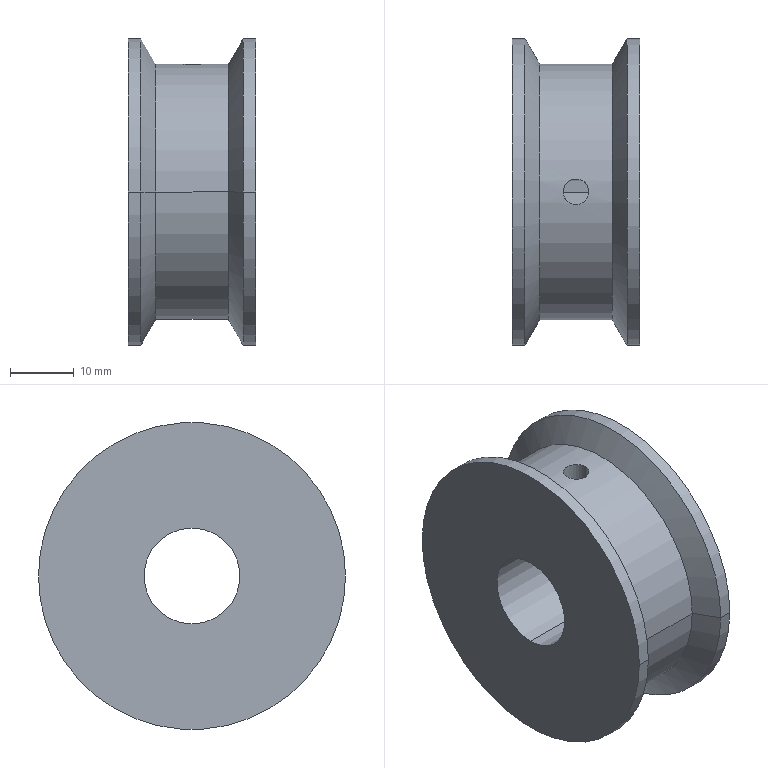Part | SolidWorks | features BaseBody 1 | 1 solid | 16 faces | box 20 x 48 x 48 mm | volume 24891 mm3 | cylinder 10 | cone 4 | plane 2 | commonest cylinder face diameters 48 x4 4 x2 15 x2 40 x2
STEP:
#1=CARTESIAN_POINT('',(2.,0.,7.5));
#2=VERTEX_POINT('',#1);
#3=CARTESIAN_POINT('',(-2.,0.,7.5));
#4=VERTEX_POINT('',#3);
#5=CARTESIAN_POINT('',(2.,0.,7.5));
#6=CARTESIAN_POINT('',(2.,0.1327,7.5));
#7=CARTESIAN_POINT('',(1.987,0.2632,7.496));
#8=CARTESIAN_POINT('',(1.936,0.5196,7.483));
#9=CARTESIAN_POINT('',(1.897,0.6469,7.473));
#10=CARTESIAN_POINT('',(1.796,0.8888,7.448));
#11=CARTESIAN_POINT('',(1.735,1.003,7.433));
#12=CARTESIAN_POINT('',(1.59,1.22,7.401));
#13=CARTESIAN_POINT('',(1.506,1.323,7.383));
#14=CARTESIAN_POINT('',(1.231,1.598,7.33));
#15=CARTESIAN_POINT('',(1.009,1.747,7.295));
#16=CARTESIAN_POINT('',(0.6481,1.897,7.256));
#17=CARTESIAN_POINT('',(0.5215,1.935,7.246));
#18=CARTESIAN_POINT('',(0.2631,1.987,7.232));
#19=CARTESIAN_POINT('',(0.1329,2.,7.228));
#20=CARTESIAN_POINT('',(-0.1292,2.,7.228));
#21=CARTESIAN_POINT('',(-0.2624,1.987,7.232));
#22=CARTESIAN_POINT('',(-0.5194,1.936,7.246));
#23=CARTESIAN_POINT('',(-0.6443,1.898,7.256));
#24=CARTESIAN_POINT('',(-1.009,1.747,7.294));
#25=CARTESIAN_POINT('',(-1.228,1.6,7.33));
#26=CARTESIAN_POINT('',(-1.506,1.322,7.383));
#27=CARTESIAN_POINT('',(-1.588,1.222,7.401));
#28=CARTESIAN_POINT('',(-1.733,1.006,7.433));
#29=CARTESIAN_POINT('',(-1.796,0.8891,7.448));
#30=CARTESIAN_POINT('',(-1.897,0.6479,7.473));
#31=CARTESIAN_POINT('',(-1.935,0.5233,7.483));
#32=CARTESIAN_POINT('',(-1.987,0.2656,7.496));
#33=CARTESIAN_POINT('',(-2.,0.1328,7.5));
#34=CARTESIAN_POINT('',(-2.,0.,7.5));
#35=B_SPLINE_CURVE_WITH_KNOTS('',3,(#5,#6,#7,#8,#9,#10,#11,#12,#13,#14,#15,#16,#17,#18,#19,#20,#21,#22,#23,#24,#25,#26,#27,#28,#29,#30,#31,#32,#33,#34),.UNSPECIFIED.,.F.,.F.,(4,2,2,2,2,2,2,2,2,2,2,2,2,2,4),(0.,0.0003925,0.0007849,0.001177,0.00157,0.002355,0.002747,0.00314,0.003532,0.003925,0.00471,0.005102,0.005495,0.005887,0.006279),.UNSPECIFIED.);
#36=EDGE_CURVE('',#2,#4,#35,.T.);
#37=ORIENTED_EDGE('',*,*,#36,.F.);
#38=CARTESIAN_POINT('',(2.,0.,20.));
#39=VERTEX_POINT('',#38);
#40=CARTESIAN_POINT('',(2.,0.,20.));
#41=DIRECTION('',(0.,0.,1.));
#42=VECTOR('',#41,1000.);
#43=LINE('',#40,#42);
#44=EDGE_CURVE('',#2,#39,#43,.T.);
#45=ORIENTED_EDGE('',*,*,#44,.T.);
#46=CARTESIAN_POINT('',(-2.,0.,20.));
#47=VERTEX_POINT('',#46);
#48=CARTESIAN_POINT('',(-2.,0.,20.));
#49=CARTESIAN_POINT('',(-2.,0.1322,20.));
#50=CARTESIAN_POINT('',(-1.987,0.2622,19.999));
#51=CARTESIAN_POINT('',(-1.936,0.5179,19.994));
#52=CARTESIAN_POINT('',(-1.898,0.6449,19.99));
#53=CARTESIAN_POINT('',(-1.797,0.8871,19.981));
#54=CARTESIAN_POINT('',(-1.736,1.002,19.975));
#55=CARTESIAN_POINT('',(-1.591,1.219,19.963));
#56=CARTESIAN_POINT('',(-1.506,1.322,19.956));
#57=CARTESIAN_POINT('',(-1.23,1.599,19.937));
#58=CARTESIAN_POINT('',(-1.007,1.748,19.924));
#59=CARTESIAN_POINT('',(-0.5257,1.947,19.905));
#60=CARTESIAN_POINT('',(-0.2624,2.,19.9));
#61=CARTESIAN_POINT('',(0.1291,2.,19.9));
#62=CARTESIAN_POINT('',(0.2617,1.987,19.901));
#63=CARTESIAN_POINT('',(0.5182,1.936,19.906));
#64=CARTESIAN_POINT('',(0.6429,1.898,19.91));
#65=CARTESIAN_POINT('',(0.8851,1.798,19.919));
#66=CARTESIAN_POINT('',(1.002,1.736,19.925));
#67=CARTESIAN_POINT('',(1.219,1.591,19.937));
#68=CARTESIAN_POINT('',(1.32,1.508,19.943));
#69=CARTESIAN_POINT('',(1.507,1.322,19.956));
#70=CARTESIAN_POINT('',(1.589,1.221,19.963));
#71=CARTESIAN_POINT('',(1.734,1.005,19.975));
#72=CARTESIAN_POINT('',(1.797,0.8877,19.981));
#73=CARTESIAN_POINT('',(1.897,0.6455,19.99));
#74=CARTESIAN_POINT('',(1.935,0.5209,19.994));
#75=CARTESIAN_POINT('',(1.987,0.2645,19.999));
#76=CARTESIAN_POINT('',(2.,0.1322,20.));
#77=CARTESIAN_POINT('',(2.,0.,20.));
#78=B_SPLINE_CURVE_WITH_KNOTS('',3,(#48,#49,#50,#51,#52,#53,#54,#55,#56,#57,#58,#59,#60,#61,#62,#63,#64,#65,#66,#67,#68,#69,#70,#71,#72,#73,#74,#75,#76,#77),.UNSPECIFIED.,.F.,.F.,(4,2,2,2,2,2,2,2,2,2,2,2,2,2,4),(0.,0.000391,0.0007819,0.001173,0.001564,0.002346,0.003128,0.003519,0.00391,0.004301,0.004692,0.005083,0.005474,0.005864,0.006255),.UNSPECIFIED.);
#79=EDGE_CURVE('',#47,#39,#78,.T.);
#80=ORIENTED_EDGE('',*,*,#79,.F.);
#81=CARTESIAN_POINT('',(-2.,0.,20.));
#82=DIRECTION('',(0.,0.,1.));
#83=VECTOR('',#82,1000.);
#84=LINE('',#81,#83);
#85=EDGE_CURVE('',#4,#47,#84,.T.);
#86=ORIENTED_EDGE('',*,*,#85,.F.);
#87=EDGE_LOOP('',(#37,#45,#80,#86));
#88=FACE_OUTER_BOUND('',#87,.T.);
#89=CARTESIAN_POINT('',(0.,0.,20.));
#90=DIRECTION('',(0.,0.,1.));
#91=DIRECTION('',(-1.,0.,0.));
#92=AXIS2_PLACEMENT_3D('',#89,#90,#91);
#93=CYLINDRICAL_SURFACE('',#92,2.);
#94=ADVANCED_FACE('',(#88),#93,.F.);
#95=CARTESIAN_POINT('',(-10.,0.,-7.5));
#96=VERTEX_POINT('',#95);
#97=CARTESIAN_POINT('',(-10.,0.,7.5));
#98=VERTEX_POINT('',#97);
#99=CARTESIAN_POINT('',(-10.,0.,0.));
#100=DIRECTION('',(1.,0.,0.));
#101=DIRECTION('',(0.,0.,1.));
#102=AXIS2_PLACEMENT_3D('',#99,#100,#101);
#103=CIRCLE('',#102,7.5);
#104=EDGE_CURVE('',#96,#98,#103,.T.);
#105=ORIENTED_EDGE('',*,*,#104,.F.);
#106=CARTESIAN_POINT('',(10.,0.,-7.5));
#107=VERTEX_POINT('',#106);
#108=CARTESIAN_POINT('',(10.,0.,-7.5));
#109=DIRECTION('',(1.,0.,0.));
#110=VECTOR('',#109,1000.);
#111=LINE('',#108,#110);
#112=EDGE_CURVE('',#96,#107,#111,.T.);
#113=ORIENTED_EDGE('',*,*,#112,.T.);
#114=CARTESIAN_POINT('',(10.,0.,7.5));
#115=VERTEX_POINT('',#114);
#116=CARTESIAN_POINT('',(10.,0.,0.));
#117=DIRECTION('',(-1.,0.,0.));
#118=DIRECTION('',(0.,0.,1.));
#119=AXIS2_PLACEMENT_3D('',#116,#117,#118);
#120=CIRCLE('',#119,7.5);
#121=EDGE_CURVE('',#115,#107,#120,.T.);
#122=ORIENTED_EDGE('',*,*,#121,.F.);
#123=CARTESIAN_POINT('',(10.,0.,7.5));
#124=DIRECTION('',(1.,0.,0.));
#125=VECTOR('',#124,1000.);
#126=LINE('',#123,#125);
#127=EDGE_CURVE('',#2,#115,#126,.T.);
#128=ORIENTED_EDGE('',*,*,#127,.F.);
#129=ORIENTED_EDGE('',*,*,#36,.T.);
#130=CARTESIAN_POINT('',(10.,0.,7.5));
#131=DIRECTION('',(1.,0.,0.));
#132=VECTOR('',#131,1000.);
#133=LINE('',#130,#132);
#134=EDGE_CURVE('',#98,#4,#133,.T.);
#135=ORIENTED_EDGE('',*,*,#134,.F.);
#136=EDGE_LOOP('',(#105,#113,#122,#128,#129,#135));
#137=FACE_OUTER_BOUND('',#136,.T.);
#138=CARTESIAN_POINT('',(10.,0.,0.));
#139=DIRECTION('',(1.,0.,0.));
#140=DIRECTION('',(0.,0.,1.));
#141=AXIS2_PLACEMENT_3D('',#138,#139,#140);
#142=CYLINDRICAL_SURFACE('',#141,7.5);
#143=ADVANCED_FACE('',(#137),#142,.F.);
#144=CARTESIAN_POINT('',(-8.,-24.,0.));
#145=VERTEX_POINT('',#144);
#146=CARTESIAN_POINT('',(-8.,24.,0.));
#147=VERTEX_POINT('',#146);
#148=CARTESIAN_POINT('',(-8.,0.,0.));
#149=DIRECTION('',(1.,0.,0.));
#150=DIRECTION('',(0.,0.,-1.));
#151=AXIS2_PLACEMENT_3D('',#148,#149,#150);
#152=CIRCLE('',#151,24.);
#153=EDGE_CURVE('',#145,#147,#152,.T.);
#154=ORIENTED_EDGE('',*,*,#153,.F.);
#155=CARTESIAN_POINT('',(-10.,-24.,0.));
#156=VERTEX_POINT('',#155);
#157=CARTESIAN_POINT('',(-9.,-24.,0.));
#158=DIRECTION('',(-1.,0.,0.));
#159=VECTOR('',#158,1000.);
#160=LINE('',#157,#159);
#161=EDGE_CURVE('',#145,#156,#160,.T.);
#162=ORIENTED_EDGE('',*,*,#161,.T.);
#163=CARTESIAN_POINT('',(-10.,24.,0.));
#164=VERTEX_POINT('',#163);
#165=CARTESIAN_POINT('',(-10.,0.,0.));
#166=DIRECTION('',(1.,0.,0.));
#167=DIRECTION('',(0.,0.,-1.));
#168=AXIS2_PLACEMENT_3D('',#165,#166,#167);
#169=CIRCLE('',#168,24.);
#170=EDGE_CURVE('',#156,#164,#169,.T.);
#171=ORIENTED_EDGE('',*,*,#170,.T.);
#172=CARTESIAN_POINT('',(-9.,24.,0.));
#173=DIRECTION('',(-1.,0.,0.));
#174=VECTOR('',#173,1000.);
#175=LINE('',#172,#174);
#176=EDGE_CURVE('',#147,#164,#175,.T.);
#177=ORIENTED_EDGE('',*,*,#176,.F.);
#178=EDGE_LOOP('',(#154,#162,#171,#177));
#179=FACE_OUTER_BOUND('',#178,.T.);
#180=CARTESIAN_POINT('',(-9.,0.,0.));
#181=DIRECTION('',(-1.,0.,0.));
#182=DIRECTION('',(0.,1.,0.));
#183=AXIS2_PLACEMENT_3D('',#180,#181,#182);
#184=CYLINDRICAL_SURFACE('',#183,24.);
#185=ADVANCED_FACE('',(#179),#184,.T.);
#186=CARTESIAN_POINT('',(-5.691,-20.,0.));
#187=VERTEX_POINT('',#186);
#188=CARTESIAN_POINT('',(-5.691,20.,0.));
#189=VERTEX_POINT('',#188);
#190=CARTESIAN_POINT('',(-5.691,0.,0.));
#191=DIRECTION('',(1.,0.,0.));
#192=DIRECTION('',(0.,0.,-1.));
#193=AXIS2_PLACEMENT_3D('',#190,#191,#192);
#194=CIRCLE('',#193,20.);
#195=EDGE_CURVE('',#187,#189,#194,.T.);
#196=ORIENTED_EDGE('',*,*,#195,.F.);
#197=CARTESIAN_POINT('',(-6.845,-22.,0.));
#198=DIRECTION('',(-0.5,-0.866,0.));
#199=VECTOR('',#198,1000.);
#200=LINE('',#197,#199);
#201=EDGE_CURVE('',#187,#145,#200,.T.);
#202=ORIENTED_EDGE('',*,*,#201,.T.);
#203=ORIENTED_EDGE('',*,*,#153,.T.);
#204=CARTESIAN_POINT('',(-6.845,22.,0.));
#205=DIRECTION('',(-0.5,0.866,0.));
#206=VECTOR('',#205,1000.);
#207=LINE('',#204,#206);
#208=EDGE_CURVE('',#189,#147,#207,.T.);
#209=ORIENTED_EDGE('',*,*,#208,.F.);
#210=EDGE_LOOP('',(#196,#202,#203,#209));
#211=FACE_OUTER_BOUND('',#210,.T.);
#212=CARTESIAN_POINT('',(-6.845,0.,0.));
#213=DIRECTION('',(-1.,0.,0.));
#214=DIRECTION('',(0.,1.,0.));
#215=AXIS2_PLACEMENT_3D('',#212,#213,#214);
#216=CONICAL_SURFACE('',#215,22.,1.047);
#217=ADVANCED_FACE('',(#211),#216,.T.);
#218=CARTESIAN_POINT('',(5.691,-20.,0.));
#219=VERTEX_POINT('',#218);
#220=CARTESIAN_POINT('',(5.691,20.,0.));
#221=VERTEX_POINT('',#220);
#222=CARTESIAN_POINT('',(5.691,0.,0.));
#223=DIRECTION('',(1.,0.,0.));
#224=DIRECTION('',(0.,0.,-1.));
#225=AXIS2_PLACEMENT_3D('',#222,#223,#224);
#226=CIRCLE('',#225,20.);
#227=EDGE_CURVE('',#219,#221,#226,.T.);
#228=ORIENTED_EDGE('',*,*,#227,.F.);
#229=CARTESIAN_POINT('',(0.,-20.,0.));
#230=DIRECTION('',(-1.,0.,0.));
#231=VECTOR('',#230,1000.);
#232=LINE('',#229,#231);
#233=EDGE_CURVE('',#219,#187,#232,.T.);
#234=ORIENTED_EDGE('',*,*,#233,.T.);
#235=ORIENTED_EDGE('',*,*,#195,.T.);
#236=CARTESIAN_POINT('',(0.,20.,0.));
#237=DIRECTION('',(-1.,0.,0.));
#238=VECTOR('',#237,1000.);
#239=LINE('',#236,#238);
#240=EDGE_CURVE('',#221,#189,#239,.T.);
#241=ORIENTED_EDGE('',*,*,#240,.F.);
#242=EDGE_LOOP('',(#228,#234,#235,#241));
#243=FACE_OUTER_BOUND('',#242,.T.);
#244=CARTESIAN_POINT('',(0.,0.,0.));
#245=DIRECTION('',(-1.,0.,0.));
#246=DIRECTION('',(0.,1.,0.));
#247=AXIS2_PLACEMENT_3D('',#244,#245,#246);
#248=CYLINDRICAL_SURFACE('',#247,20.);
#249=ADVANCED_FACE('',(#243),#248,.T.);
#250=CARTESIAN_POINT('',(5.691,0.,0.));
#251=DIRECTION('',(1.,0.,0.));
#252=DIRECTION('',(0.,0.,-1.));
#253=AXIS2_PLACEMENT_3D('',#250,#251,#252);
#254=CIRCLE('',#253,20.);
#255=EDGE_CURVE('',#221,#219,#254,.T.);
#256=ORIENTED_EDGE('',*,*,#255,.T.);
#257=CARTESIAN_POINT('',(8.,-24.,0.));
#258=VERTEX_POINT('',#257);
#259=CARTESIAN_POINT('',(6.845,-22.,0.));
#260=DIRECTION('',(0.5,-0.866,0.));
#261=VECTOR('',#260,1000.);
#262=LINE('',#259,#261);
#263=EDGE_CURVE('',#219,#258,#262,.T.);
#264=ORIENTED_EDGE('',*,*,#263,.T.);
#265=CARTESIAN_POINT('',(8.,24.,0.));
#266=VERTEX_POINT('',#265);
#267=CARTESIAN_POINT('',(8.,0.,0.));
#268=DIRECTION('',(1.,0.,0.));
#269=DIRECTION('',(0.,0.,-1.));
#270=AXIS2_PLACEMENT_3D('',#267,#268,#269);
#271=CIRCLE('',#270,24.);
#272=EDGE_CURVE('',#266,#258,#271,.T.);
#273=ORIENTED_EDGE('',*,*,#272,.F.);
#274=CARTESIAN_POINT('',(6.845,22.,0.));
#275=DIRECTION('',(0.5,0.866,0.));
#276=VECTOR('',#275,1000.);
#277=LINE('',#274,#276);
#278=EDGE_CURVE('',#221,#266,#277,.T.);
#279=ORIENTED_EDGE('',*,*,#278,.F.);
#280=EDGE_LOOP('',(#256,#264,#273,#279));
#281=FACE_OUTER_BOUND('',#280,.T.);
#282=CARTESIAN_POINT('',(6.845,0.,0.));
#283=DIRECTION('',(1.,0.,0.));
#284=DIRECTION('',(0.,1.,0.));
#285=AXIS2_PLACEMENT_3D('',#282,#283,#284);
#286=CONICAL_SURFACE('',#285,22.,1.047);
#287=ADVANCED_FACE('',(#281),#286,.T.);
#288=CARTESIAN_POINT('',(10.,-24.,0.));
#289=VERTEX_POINT('',#288);
#290=CARTESIAN_POINT('',(10.,24.,0.));
#291=VERTEX_POINT('',#290);
#292=CARTESIAN_POINT('',(10.,0.,0.));
#293=DIRECTION('',(1.,0.,0.));
#294=DIRECTION('',(0.,0.,-1.));
#295=AXIS2_PLACEMENT_3D('',#292,#293,#294);
#296=CIRCLE('',#295,24.);
#297=EDGE_CURVE('',#289,#291,#296,.T.);
#298=ORIENTED_EDGE('',*,*,#297,.F.);
#299=CARTESIAN_POINT('',(9.,-24.,0.));
#300=DIRECTION('',(-1.,0.,0.));
#301=VECTOR('',#300,1000.);
#302=LINE('',#299,#301);
#303=EDGE_CURVE('',#289,#258,#302,.T.);
#304=ORIENTED_EDGE('',*,*,#303,.T.);
#305=CARTESIAN_POINT('',(8.,0.,0.));
#306=DIRECTION('',(1.,0.,0.));
#307=DIRECTION('',(0.,0.,-1.));
#308=AXIS2_PLACEMENT_3D('',#305,#306,#307);
#309=CIRCLE('',#308,24.);
#310=EDGE_CURVE('',#258,#266,#309,.T.);
#311=ORIENTED_EDGE('',*,*,#310,.T.);
#312=CARTESIAN_POINT('',(9.,24.,0.));
#313=DIRECTION('',(-1.,0.,0.));
#314=VECTOR('',#313,1000.);
#315=LINE('',#312,#314);
#316=EDGE_CURVE('',#291,#266,#315,.T.);
#317=ORIENTED_EDGE('',*,*,#316,.F.);
#318=EDGE_LOOP('',(#298,#304,#311,#317));
#319=FACE_OUTER_BOUND('',#318,.T.);
#320=CARTESIAN_POINT('',(9.,0.,0.));
#321=DIRECTION('',(-1.,0.,0.));
#322=DIRECTION('',(0.,1.,0.));
#323=AXIS2_PLACEMENT_3D('',#320,#321,#322);
#324=CYLINDRICAL_SURFACE('',#323,24.);
#325=ADVANCED_FACE('',(#319),#324,.T.);
#326=CARTESIAN_POINT('',(-10.,0.,0.));
#327=DIRECTION('',(1.,0.,0.));
#328=DIRECTION('',(0.,0.,1.));
#329=AXIS2_PLACEMENT_3D('',#326,#327,#328);
#330=CIRCLE('',#329,7.5);
#331=EDGE_CURVE('',#98,#96,#330,.T.);
#332=ORIENTED_EDGE('',*,*,#331,.T.);
#333=ORIENTED_EDGE('',*,*,#104,.T.);
#334=EDGE_LOOP('',(#332,#333));
#335=FACE_BOUND('',#334,.T.);
#336=CARTESIAN_POINT('',(-10.,0.,0.));
#337=DIRECTION('',(1.,0.,0.));
#338=DIRECTION('',(0.,0.,-1.));
#339=AXIS2_PLACEMENT_3D('',#336,#337,#338);
#340=CIRCLE('',#339,24.);
#341=EDGE_CURVE('',#164,#156,#340,.T.);
#342=ORIENTED_EDGE('',*,*,#341,.F.);
#343=ORIENTED_EDGE('',*,*,#170,.F.);
#344=EDGE_LOOP('',(#342,#343));
#345=FACE_OUTER_BOUND('',#344,.T.);
#346=CARTESIAN_POINT('',(-10.,24.,0.));
#347=DIRECTION('',(-1.,0.,0.));
#348=DIRECTION('',(0.,0.,1.));
#349=AXIS2_PLACEMENT_3D('',#346,#347,#348);
#350=PLANE('',#349);
#351=ADVANCED_FACE('',(#335,#345),#350,.T.);
#352=ORIENTED_EDGE('',*,*,#121,.T.);
#353=CARTESIAN_POINT('',(10.,0.,0.));
#354=DIRECTION('',(-1.,0.,0.));
#355=DIRECTION('',(0.,0.,1.));
#356=AXIS2_PLACEMENT_3D('',#353,#354,#355);
#357=CIRCLE('',#356,7.5);
#358=EDGE_CURVE('',#107,#115,#357,.T.);
#359=ORIENTED_EDGE('',*,*,#358,.T.);
#360=EDGE_LOOP('',(#352,#359));
#361=FACE_BOUND('',#360,.T.);
#362=CARTESIAN_POINT('',(10.,0.,0.));
#363=DIRECTION('',(1.,0.,0.));
#364=DIRECTION('',(0.,0.,-1.));
#365=AXIS2_PLACEMENT_3D('',#362,#363,#364);
#366=CIRCLE('',#365,24.);
#367=EDGE_CURVE('',#291,#289,#366,.T.);
#368=ORIENTED_EDGE('',*,*,#367,.T.);
#369=ORIENTED_EDGE('',*,*,#297,.T.);
#370=EDGE_LOOP('',(#368,#369));
#371=FACE_OUTER_BOUND('',#370,.T.);
#372=CARTESIAN_POINT('',(10.,0.,0.));
#373=DIRECTION('',(1.,0.,0.));
#374=DIRECTION('',(0.,1.,0.));
#375=AXIS2_PLACEMENT_3D('',#372,#373,#374);
#376=PLANE('',#375);
#377=ADVANCED_FACE('',(#361,#371),#376,.T.);
#378=ORIENTED_EDGE('',*,*,#303,.F.);
#379=ORIENTED_EDGE('',*,*,#367,.F.);
#380=ORIENTED_EDGE('',*,*,#316,.T.);
#381=ORIENTED_EDGE('',*,*,#272,.T.);
#382=EDGE_LOOP('',(#378,#379,#380,#381));
#383=FACE_OUTER_BOUND('',#382,.T.);
#384=CARTESIAN_POINT('',(9.,0.,0.));
#385=DIRECTION('',(-1.,0.,0.));
#386=DIRECTION('',(0.,1.,0.));
#387=AXIS2_PLACEMENT_3D('',#384,#385,#386);
#388=CYLINDRICAL_SURFACE('',#387,24.);
#389=ADVANCED_FACE('',(#383),#388,.T.);
#390=ORIENTED_EDGE('',*,*,#263,.F.);
#391=ORIENTED_EDGE('',*,*,#227,.T.);
#392=ORIENTED_EDGE('',*,*,#278,.T.);
#393=ORIENTED_EDGE('',*,*,#310,.F.);
#394=EDGE_LOOP('',(#390,#391,#392,#393));
#395=FACE_OUTER_BOUND('',#394,.T.);
#396=CARTESIAN_POINT('',(6.845,0.,0.));
#397=DIRECTION('',(1.,0.,0.));
#398=DIRECTION('',(0.,1.,0.));
#399=AXIS2_PLACEMENT_3D('',#396,#397,#398);
#400=CONICAL_SURFACE('',#399,22.,1.047);
#401=ADVANCED_FACE('',(#395),#400,.T.);
#402=ORIENTED_EDGE('',*,*,#233,.F.);
#403=ORIENTED_EDGE('',*,*,#255,.F.);
#404=ORIENTED_EDGE('',*,*,#240,.T.);
#405=CARTESIAN_POINT('',(-5.691,0.,0.));
#406=DIRECTION('',(1.,0.,0.));
#407=DIRECTION('',(0.,0.,-1.));
#408=AXIS2_PLACEMENT_3D('',#405,#406,#407);
#409=CIRCLE('',#408,20.);
#410=EDGE_CURVE('',#189,#187,#409,.T.);
#411=ORIENTED_EDGE('',*,*,#410,.T.);
#412=EDGE_LOOP('',(#402,#403,#404,#411));
#413=FACE_OUTER_BOUND('',#412,.T.);
#414=ORIENTED_EDGE('',*,*,#79,.T.);
#415=CARTESIAN_POINT('',(2.,0.,20.));
#416=CARTESIAN_POINT('',(2.,-0.1322,20.));
#417=CARTESIAN_POINT('',(1.987,-0.2622,19.999));
#418=CARTESIAN_POINT('',(1.936,-0.5179,19.994));
#419=CARTESIAN_POINT('',(1.898,-0.6449,19.99));
#420=CARTESIAN_POINT('',(1.797,-0.8871,19.981));
#421=CARTESIAN_POINT('',(1.736,-1.002,19.975));
#422=CARTESIAN_POINT('',(1.591,-1.219,19.963));
#423=CARTESIAN_POINT('',(1.506,-1.322,19.956));
#424=CARTESIAN_POINT('',(1.23,-1.599,19.937));
#425=CARTESIAN_POINT('',(1.007,-1.748,19.924));
#426=CARTESIAN_POINT('',(0.5257,-1.947,19.905));
#427=CARTESIAN_POINT('',(0.2624,-2.,19.9));
#428=CARTESIAN_POINT('',(-0.1291,-2.,19.9));
#429=CARTESIAN_POINT('',(-0.2617,-1.987,19.901));
#430=CARTESIAN_POINT('',(-0.5182,-1.936,19.906));
#431=CARTESIAN_POINT('',(-0.6429,-1.898,19.91));
#432=CARTESIAN_POINT('',(-0.8851,-1.798,19.919));
#433=CARTESIAN_POINT('',(-1.002,-1.736,19.925));
#434=CARTESIAN_POINT('',(-1.219,-1.591,19.937));
#435=CARTESIAN_POINT('',(-1.32,-1.508,19.943));
#436=CARTESIAN_POINT('',(-1.507,-1.322,19.956));
#437=CARTESIAN_POINT('',(-1.589,-1.221,19.963));
#438=CARTESIAN_POINT('',(-1.734,-1.005,19.975));
#439=CARTESIAN_POINT('',(-1.797,-0.8877,19.981));
#440=CARTESIAN_POINT('',(-1.897,-0.6455,19.99));
#441=CARTESIAN_POINT('',(-1.935,-0.5209,19.994));
#442=CARTESIAN_POINT('',(-1.987,-0.2645,19.999));
#443=CARTESIAN_POINT('',(-2.,-0.1322,20.));
#444=CARTESIAN_POINT('',(-2.,0.,20.));
#445=B_SPLINE_CURVE_WITH_KNOTS('',3,(#415,#416,#417,#418,#419,#420,#421,#422,#423,#424,#425,#426,#427,#428,#429,#430,#431,#432,#433,#434,#435,#436,#437,#438,#439,#440,#441,#442,#443,#444),.UNSPECIFIED.,.F.,.F.,(4,2,2,2,2,2,2,2,2,2,2,2,2,2,4),(0.006255,0.006646,0.007037,0.007428,0.007819,0.008601,0.009383,0.009774,0.01017,0.01056,0.01095,0.01134,0.01173,0.01212,0.01251),.UNSPECIFIED.);
#446=EDGE_CURVE('',#39,#47,#445,.T.);
#447=ORIENTED_EDGE('',*,*,#446,.T.);
#448=EDGE_LOOP('',(#414,#447));
#449=FACE_BOUND('',#448,.T.);
#450=CARTESIAN_POINT('',(0.,0.,0.));
#451=DIRECTION('',(-1.,0.,0.));
#452=DIRECTION('',(0.,1.,0.));
#453=AXIS2_PLACEMENT_3D('',#450,#451,#452);
#454=CYLINDRICAL_SURFACE('',#453,20.);
#455=ADVANCED_FACE('',(#413,#449),#454,.T.);
#456=ORIENTED_EDGE('',*,*,#201,.F.);
#457=ORIENTED_EDGE('',*,*,#410,.F.);
#458=ORIENTED_EDGE('',*,*,#208,.T.);
#459=CARTESIAN_POINT('',(-8.,0.,0.));
#460=DIRECTION('',(1.,0.,0.));
#461=DIRECTION('',(0.,0.,-1.));
#462=AXIS2_PLACEMENT_3D('',#459,#460,#461);
#463=CIRCLE('',#462,24.);
#464=EDGE_CURVE('',#147,#145,#463,.T.);
#465=ORIENTED_EDGE('',*,*,#464,.T.);
#466=EDGE_LOOP('',(#456,#457,#458,#465));
#467=FACE_OUTER_BOUND('',#466,.T.);
#468=CARTESIAN_POINT('',(-6.845,0.,0.));
#469=DIRECTION('',(-1.,0.,0.));
#470=DIRECTION('',(0.,1.,0.));
#471=AXIS2_PLACEMENT_3D('',#468,#469,#470);
#472=CONICAL_SURFACE('',#471,22.,1.047);
#473=ADVANCED_FACE('',(#467),#472,.T.);
#474=ORIENTED_EDGE('',*,*,#161,.F.);
#475=ORIENTED_EDGE('',*,*,#464,.F.);
#476=ORIENTED_EDGE('',*,*,#176,.T.);
#477=ORIENTED_EDGE('',*,*,#341,.T.);
#478=EDGE_LOOP('',(#474,#475,#476,#477));
#479=FACE_OUTER_BOUND('',#478,.T.);
#480=CARTESIAN_POINT('',(-9.,0.,0.));
#481=DIRECTION('',(-1.,0.,0.));
#482=DIRECTION('',(0.,1.,0.));
#483=AXIS2_PLACEMENT_3D('',#480,#481,#482);
#484=CYLINDRICAL_SURFACE('',#483,24.);
#485=ADVANCED_FACE('',(#479),#484,.T.);
#486=ORIENTED_EDGE('',*,*,#112,.F.);
#487=ORIENTED_EDGE('',*,*,#331,.F.);
#488=ORIENTED_EDGE('',*,*,#134,.T.);
#489=CARTESIAN_POINT('',(-2.,0.,7.5));
#490=CARTESIAN_POINT('',(-2.,-0.1327,7.5));
#491=CARTESIAN_POINT('',(-1.987,-0.2632,7.496));
#492=CARTESIAN_POINT('',(-1.936,-0.5196,7.483));
#493=CARTESIAN_POINT('',(-1.897,-0.6469,7.473));
#494=CARTESIAN_POINT('',(-1.796,-0.8888,7.448));
#495=CARTESIAN_POINT('',(-1.735,-1.003,7.433));
#496=CARTESIAN_POINT('',(-1.59,-1.22,7.401));
#497=CARTESIAN_POINT('',(-1.506,-1.323,7.383));
#498=CARTESIAN_POINT('',(-1.231,-1.598,7.33));
#499=CARTESIAN_POINT('',(-1.009,-1.747,7.295));
#500=CARTESIAN_POINT('',(-0.6481,-1.897,7.256));
#501=CARTESIAN_POINT('',(-0.5215,-1.935,7.246));
#502=CARTESIAN_POINT('',(-0.2631,-1.987,7.232));
#503=CARTESIAN_POINT('',(-0.1329,-2.,7.228));
#504=CARTESIAN_POINT('',(0.1292,-2.,7.228));
#505=CARTESIAN_POINT('',(0.2624,-1.987,7.232));
#506=CARTESIAN_POINT('',(0.5194,-1.936,7.246));
#507=CARTESIAN_POINT('',(0.6443,-1.898,7.256));
#508=CARTESIAN_POINT('',(1.009,-1.747,7.294));
#509=CARTESIAN_POINT('',(1.228,-1.6,7.33));
#510=CARTESIAN_POINT('',(1.506,-1.322,7.383));
#511=CARTESIAN_POINT('',(1.588,-1.222,7.401));
#512=CARTESIAN_POINT('',(1.733,-1.006,7.433));
#513=CARTESIAN_POINT('',(1.796,-0.8891,7.448));
#514=CARTESIAN_POINT('',(1.897,-0.6479,7.473));
#515=CARTESIAN_POINT('',(1.935,-0.5233,7.483));
#516=CARTESIAN_POINT('',(1.987,-0.2656,7.496));
#517=CARTESIAN_POINT('',(2.,-0.1327,7.5));
#518=CARTESIAN_POINT('',(2.,0.,7.5));
#519=B_SPLINE_CURVE_WITH_KNOTS('',3,(#489,#490,#491,#492,#493,#494,#495,#496,#497,#498,#499,#500,#501,#502,#503,#504,#505,#506,#507,#508,#509,#510,#511,#512,#513,#514,#515,#516,#517,#518),.UNSPECIFIED.,.F.,.F.,(4,2,2,2,2,2,2,2,2,2,2,2,2,2,4),(0.006279,0.006672,0.007064,0.007457,0.007849,0.008634,0.009027,0.009419,0.009811,0.0102,0.01099,0.01138,0.01177,0.01217,0.01256),.UNSPECIFIED.);
#520=EDGE_CURVE('',#4,#2,#519,.T.);
#521=ORIENTED_EDGE('',*,*,#520,.T.);
#522=ORIENTED_EDGE('',*,*,#127,.T.);
#523=ORIENTED_EDGE('',*,*,#358,.F.);
#524=EDGE_LOOP('',(#486,#487,#488,#521,#522,#523));
#525=FACE_OUTER_BOUND('',#524,.T.);
#526=CARTESIAN_POINT('',(10.,0.,0.));
#527=DIRECTION('',(1.,0.,0.));
#528=DIRECTION('',(0.,0.,1.));
#529=AXIS2_PLACEMENT_3D('',#526,#527,#528);
#530=CYLINDRICAL_SURFACE('',#529,7.5);
#531=ADVANCED_FACE('',(#525),#530,.F.);
#532=ORIENTED_EDGE('',*,*,#44,.F.);
#533=ORIENTED_EDGE('',*,*,#520,.F.);
#534=ORIENTED_EDGE('',*,*,#85,.T.);
#535=ORIENTED_EDGE('',*,*,#446,.F.);
#536=EDGE_LOOP('',(#532,#533,#534,#535));
#537=FACE_OUTER_BOUND('',#536,.T.);
#538=CARTESIAN_POINT('',(0.,0.,20.));
#539=DIRECTION('',(0.,0.,1.));
#540=DIRECTION('',(-1.,0.,0.));
#541=AXIS2_PLACEMENT_3D('',#538,#539,#540);
#542=CYLINDRICAL_SURFACE('',#541,2.);
#543=ADVANCED_FACE('',(#537),#542,.F.);
#544=CLOSED_SHELL('',(#94,#143,#185,#217,#249,#287,#325,#351,#377,#389,#401,#455,#473,#485,#531,#543));
#545=MANIFOLD_SOLID_BREP('',#544);
#546=CARTESIAN_POINT('',(0.,0.,0.));
#547=DIRECTION('',(0.,0.,1.));
#548=DIRECTION('',(1.,0.,0.));
#549=AXIS2_PLACEMENT_3D('',#546,#547,#548);
#550=(LENGTH_UNIT()NAMED_UNIT(*)SI_UNIT(.MILLI.,.METRE.));
#551=UNCERTAINTY_MEASURE_WITH_UNIT(LENGTH_MEASURE(0.00001),#550,'','');
#552=(NAMED_UNIT(*)PLANE_ANGLE_UNIT()SI_UNIT($,.RADIAN.));
#553=(NAMED_UNIT(*)SI_UNIT($,.STERADIAN.)SOLID_ANGLE_UNIT());
#554=(GEOMETRIC_REPRESENTATION_CONTEXT(3)GLOBAL_UNCERTAINTY_ASSIGNED_CONTEXT((#551))GLOBAL_UNIT_ASSIGNED_CONTEXT((#550,#552,#553))REPRESENTATION_CONTEXT('',''));
#555=ADVANCED_BREP_SHAPE_REPRESENTATION('',(#545,#549),#554);